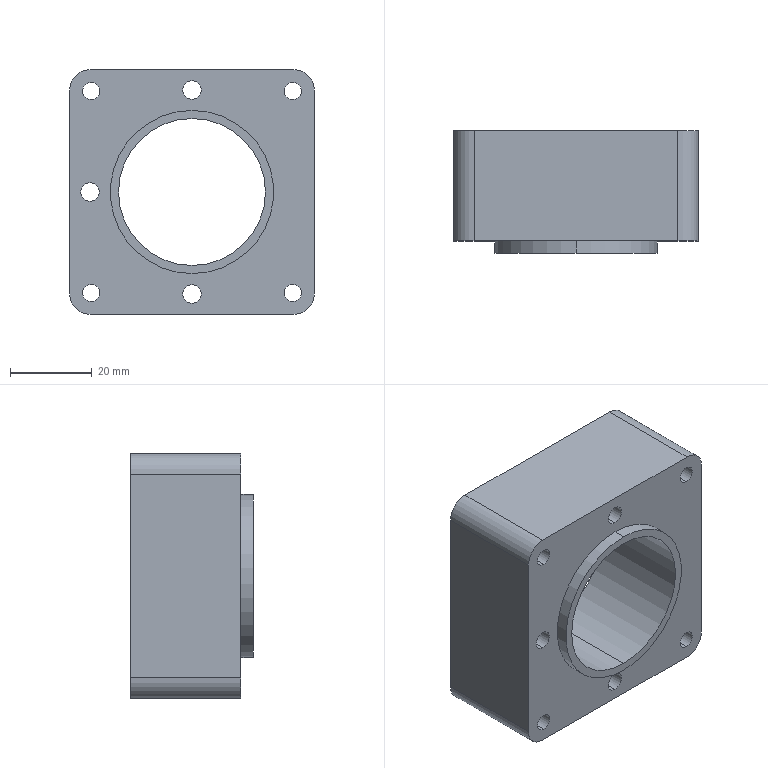Part | STEP file | lead screw 400W motor direct-connect flange | 1 solid | 45 faces | box 60 x 30 x 60 mm | volume 61401 mm3 | cylinder 31 | plane 11 | cone 3 | commonest cylinder face diameters 4.2 x8 4.5 x6 8 x6 10 x4 50 x3 36 x2